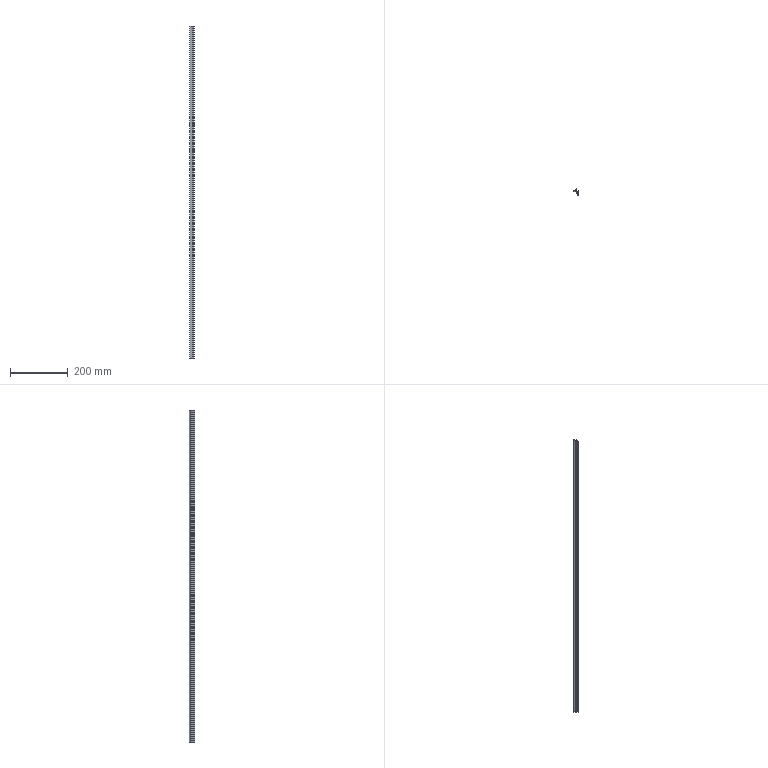Part | SolidWorks | features BaseBody 1, ICE 1, MoveFace 1 | 1 solid | 27 faces | box 14 x 20.3 x 1150 mm | volume 58553 mm3 | plane 20 | cylinder 7 | commonest cylinder face diameters 0.387 x2 0.8 x2 0.4 x1 20 x1 22 x1
STEP:
#1=CARTESIAN_POINT('',(-5.304,-0.625,200.));
#2=VERTEX_POINT('',#1);
#3=CARTESIAN_POINT('',(-5.449,-0.8125,200.));
#4=VERTEX_POINT('',#3);
#5=CARTESIAN_POINT('',(-5.255,-0.8125,200.));
#6=DIRECTION('',(0.,0.,1.));
#7=DIRECTION('',(-1.,0.,0.));
#8=AXIS2_PLACEMENT_3D('',#5,#6,#7);
#9=CIRCLE('',#8,0.1937);
#10=EDGE_CURVE('',#2,#4,#9,.T.);
#11=ORIENTED_EDGE('',*,*,#10,.T.);
#12=CARTESIAN_POINT('',(-5.449,-0.8125,-950.));
#13=VERTEX_POINT('',#12);
#14=CARTESIAN_POINT('',(-5.449,-0.8125,230.));
#15=DIRECTION('',(0.,0.,-1.));
#16=VECTOR('',#15,1000.);
#17=LINE('',#14,#16);
#18=EDGE_CURVE('',#4,#13,#17,.T.);
#19=ORIENTED_EDGE('',*,*,#18,.T.);
#20=CARTESIAN_POINT('',(-5.304,-0.625,-950.));
#21=VERTEX_POINT('',#20);
#22=CARTESIAN_POINT('',(-5.255,-0.8125,-950.));
#23=DIRECTION('',(0.,0.,-1.));
#24=DIRECTION('',(1.,0.,0.));
#25=AXIS2_PLACEMENT_3D('',#22,#23,#24);
#26=CIRCLE('',#25,0.1937);
#27=EDGE_CURVE('',#13,#21,#26,.T.);
#28=ORIENTED_EDGE('',*,*,#27,.T.);
#29=CARTESIAN_POINT('',(-5.304,-0.625,230.));
#30=DIRECTION('',(0.,0.,-1.));
#31=VECTOR('',#30,1000.);
#32=LINE('',#29,#31);
#33=EDGE_CURVE('',#2,#21,#32,.T.);
#34=ORIENTED_EDGE('',*,*,#33,.F.);
#35=EDGE_LOOP('',(#11,#19,#28,#34));
#36=FACE_OUTER_BOUND('',#35,.T.);
#37=CARTESIAN_POINT('',(-5.255,-0.8125,230.));
#38=DIRECTION('',(0.,0.,-1.));
#39=DIRECTION('',(-1.,0.,0.));
#40=AXIS2_PLACEMENT_3D('',#37,#38,#39);
#41=CYLINDRICAL_SURFACE('',#40,0.1937);
#42=ADVANCED_FACE('',(#36),#41,.F.);
#43=CARTESIAN_POINT('',(5.,-1.,-950.));
#44=VERTEX_POINT('',#43);
#45=CARTESIAN_POINT('',(5.,-14.3,-950.));
#46=VERTEX_POINT('',#45);
#47=CARTESIAN_POINT('',(5.,29.623,-950.));
#48=DIRECTION('',(0.,-1.,0.));
#49=VECTOR('',#48,1000.);
#50=LINE('',#47,#49);
#51=EDGE_CURVE('',#44,#46,#50,.T.);
#52=ORIENTED_EDGE('',*,*,#51,.F.);
#53=CARTESIAN_POINT('',(5.,-1.,200.));
#54=VERTEX_POINT('',#53);
#55=CARTESIAN_POINT('',(5.,-1.,230.));
#56=DIRECTION('',(0.,0.,-1.));
#57=VECTOR('',#56,1000.);
#58=LINE('',#55,#57);
#59=EDGE_CURVE('',#54,#44,#58,.T.);
#60=ORIENTED_EDGE('',*,*,#59,.F.);
#61=CARTESIAN_POINT('',(5.,-14.3,200.));
#62=VERTEX_POINT('',#61);
#63=CARTESIAN_POINT('',(5.,-14.3,200.));
#64=DIRECTION('',(0.,1.,0.));
#65=VECTOR('',#64,1000.);
#66=LINE('',#63,#65);
#67=EDGE_CURVE('',#62,#54,#66,.T.);
#68=ORIENTED_EDGE('',*,*,#67,.F.);
#69=CARTESIAN_POINT('',(5.,-14.3,230.));
#70=DIRECTION('',(0.,0.,1.));
#71=VECTOR('',#70,1000.);
#72=LINE('',#69,#71);
#73=EDGE_CURVE('',#46,#62,#72,.T.);
#74=ORIENTED_EDGE('',*,*,#73,.F.);
#75=EDGE_LOOP('',(#52,#60,#68,#74));
#76=FACE_OUTER_BOUND('',#75,.T.);
#77=CARTESIAN_POINT('',(5.,-14.3,230.));
#78=DIRECTION('',(-1.,0.,0.));
#79=DIRECTION('',(0.,0.,1.));
#80=AXIS2_PLACEMENT_3D('',#77,#78,#79);
#81=PLANE('',#80);
#82=ADVANCED_FACE('',(#76),#81,.F.);
#83=CARTESIAN_POINT('',(-9.,-2.,-950.));
#84=VERTEX_POINT('',#83);
#85=CARTESIAN_POINT('',(-9.,-2.,200.));
#86=VERTEX_POINT('',#85);
#87=CARTESIAN_POINT('',(-9.,-2.,230.));
#88=DIRECTION('',(0.,0.,1.));
#89=VECTOR('',#88,1000.);
#90=LINE('',#87,#89);
#91=EDGE_CURVE('',#84,#86,#90,.T.);
#92=ORIENTED_EDGE('',*,*,#91,.F.);
#93=CARTESIAN_POINT('',(0.9,-2.,-950.));
#94=VERTEX_POINT('',#93);
#95=CARTESIAN_POINT('',(5.,-2.,-950.));
#96=DIRECTION('',(-1.,0.,0.));
#97=VECTOR('',#96,1000.);
#98=LINE('',#95,#97);
#99=EDGE_CURVE('',#94,#84,#98,.T.);
#100=ORIENTED_EDGE('',*,*,#99,.F.);
#101=CARTESIAN_POINT('',(0.9,-2.,200.));
#102=VERTEX_POINT('',#101);
#103=CARTESIAN_POINT('',(0.9,-2.,230.));
#104=DIRECTION('',(0.,0.,-1.));
#105=VECTOR('',#104,1000.);
#106=LINE('',#103,#105);
#107=EDGE_CURVE('',#102,#94,#106,.T.);
#108=ORIENTED_EDGE('',*,*,#107,.F.);
#109=CARTESIAN_POINT('',(5.,-2.,200.));
#110=DIRECTION('',(1.,0.,0.));
#111=VECTOR('',#110,1000.);
#112=LINE('',#109,#111);
#113=EDGE_CURVE('',#86,#102,#112,.T.);
#114=ORIENTED_EDGE('',*,*,#113,.F.);
#115=EDGE_LOOP('',(#92,#100,#108,#114));
#116=FACE_OUTER_BOUND('',#115,.T.);
#117=CARTESIAN_POINT('',(-9.,-2.,230.));
#118=DIRECTION('',(0.,1.,0.));
#119=DIRECTION('',(0.,0.,1.));
#120=AXIS2_PLACEMENT_3D('',#117,#118,#119);
#121=PLANE('',#120);
#122=ADVANCED_FACE('',(#116),#121,.F.);
#123=CARTESIAN_POINT('',(4.,-6.,200.));
#124=VERTEX_POINT('',#123);
#125=CARTESIAN_POINT('',(4.,-3.,200.));
#126=VERTEX_POINT('',#125);
#127=CARTESIAN_POINT('',(4.,29.623,200.));
#128=DIRECTION('',(0.,1.,0.));
#129=VECTOR('',#128,1000.);
#130=LINE('',#127,#129);
#131=EDGE_CURVE('',#124,#126,#130,.T.);
#132=ORIENTED_EDGE('',*,*,#131,.F.);
#133=CARTESIAN_POINT('',(1.,-6.,200.));
#134=VERTEX_POINT('',#133);
#135=CARTESIAN_POINT('',(5.,-6.,200.));
#136=DIRECTION('',(1.,0.,0.));
#137=VECTOR('',#136,1000.);
#138=LINE('',#135,#137);
#139=EDGE_CURVE('',#134,#124,#138,.T.);
#140=ORIENTED_EDGE('',*,*,#139,.F.);
#141=CARTESIAN_POINT('',(1.,-6.7,200.));
#142=VERTEX_POINT('',#141);
#143=CARTESIAN_POINT('',(1.,-6.,200.));
#144=DIRECTION('',(0.,-1.,0.));
#145=VECTOR('',#144,1000.);
#146=LINE('',#143,#145);
#147=EDGE_CURVE('',#134,#142,#146,.T.);
#148=ORIENTED_EDGE('',*,*,#147,.T.);
#149=CARTESIAN_POINT('',(-1.7,-6.7,200.));
#150=VERTEX_POINT('',#149);
#151=CARTESIAN_POINT('',(5.,-6.7,200.));
#152=DIRECTION('',(1.,0.,0.));
#153=VECTOR('',#152,1000.);
#154=LINE('',#151,#153);
#155=EDGE_CURVE('',#150,#142,#154,.T.);
#156=ORIENTED_EDGE('',*,*,#155,.F.);
#157=CARTESIAN_POINT('',(-1.7,-7.7,200.));
#158=VERTEX_POINT('',#157);
#159=CARTESIAN_POINT('',(-1.7,-6.7,200.));
#160=DIRECTION('',(0.,-1.,0.));
#161=VECTOR('',#160,1000.);
#162=LINE('',#159,#161);
#163=EDGE_CURVE('',#150,#158,#162,.T.);
#164=ORIENTED_EDGE('',*,*,#163,.T.);
#165=CARTESIAN_POINT('',(4.,-7.7,200.));
#166=VERTEX_POINT('',#165);
#167=CARTESIAN_POINT('',(5.,-7.7,200.));
#168=DIRECTION('',(-1.,0.,0.));
#169=VECTOR('',#168,1000.);
#170=LINE('',#167,#169);
#171=EDGE_CURVE('',#166,#158,#170,.T.);
#172=ORIENTED_EDGE('',*,*,#171,.F.);
#173=CARTESIAN_POINT('',(4.,-14.3,200.));
#174=VERTEX_POINT('',#173);
#175=CARTESIAN_POINT('',(4.,29.623,200.));
#176=DIRECTION('',(0.,1.,0.));
#177=VECTOR('',#176,1000.);
#178=LINE('',#175,#177);
#179=EDGE_CURVE('',#174,#166,#178,.T.);
#180=ORIENTED_EDGE('',*,*,#179,.F.);
#181=CARTESIAN_POINT('',(5.,-14.3,200.));
#182=DIRECTION('',(-1.,0.,0.));
#183=VECTOR('',#182,1000.);
#184=LINE('',#181,#183);
#185=EDGE_CURVE('',#62,#174,#184,.T.);
#186=ORIENTED_EDGE('',*,*,#185,.F.);
#187=ORIENTED_EDGE('',*,*,#67,.T.);
#188=CARTESIAN_POINT('',(-5.207,-1.,200.));
#189=VERTEX_POINT('',#188);
#190=CARTESIAN_POINT('',(5.,-1.,200.));
#191=DIRECTION('',(1.,0.,0.));
#192=VECTOR('',#191,1000.);
#193=LINE('',#190,#192);
#194=EDGE_CURVE('',#189,#54,#193,.T.);
#195=ORIENTED_EDGE('',*,*,#194,.F.);
#196=CARTESIAN_POINT('',(-5.255,-0.8125,200.));
#197=DIRECTION('',(0.,0.,1.));
#198=DIRECTION('',(-1.,0.,0.));
#199=AXIS2_PLACEMENT_3D('',#196,#197,#198);
#200=CIRCLE('',#199,0.1937);
#201=EDGE_CURVE('',#4,#189,#200,.T.);
#202=ORIENTED_EDGE('',*,*,#201,.F.);
#203=ORIENTED_EDGE('',*,*,#10,.F.);
#204=CARTESIAN_POINT('',(-1.368,3.063,200.));
#205=VERTEX_POINT('',#204);
#206=CARTESIAN_POINT('',(-10.628,9.,200.));
#207=DIRECTION('',(0.,0.,1.));
#208=DIRECTION('',(-1.,0.,0.));
#209=AXIS2_PLACEMENT_3D('',#206,#207,#208);
#210=CIRCLE('',#209,11.);
#211=EDGE_CURVE('',#2,#205,#210,.T.);
#212=ORIENTED_EDGE('',*,*,#211,.T.);
#213=CARTESIAN_POINT('',(-1.,2.955,200.));
#214=VERTEX_POINT('',#213);
#215=CARTESIAN_POINT('',(-1.2,2.955,200.));
#216=DIRECTION('',(0.,0.,1.));
#217=DIRECTION('',(-1.,0.,0.));
#218=AXIS2_PLACEMENT_3D('',#215,#216,#217);
#219=CIRCLE('',#218,0.2);
#220=EDGE_CURVE('',#214,#205,#219,.T.);
#221=ORIENTED_EDGE('',*,*,#220,.F.);
#222=CARTESIAN_POINT('',(-1.,1.5,200.));
#223=VERTEX_POINT('',#222);
#224=CARTESIAN_POINT('',(-1.,2.955,200.));
#225=DIRECTION('',(0.,1.,0.));
#226=VECTOR('',#225,1000.);
#227=LINE('',#224,#226);
#228=EDGE_CURVE('',#223,#214,#227,.T.);
#229=ORIENTED_EDGE('',*,*,#228,.F.);
#230=CARTESIAN_POINT('',(0.,1.5,200.));
#231=VERTEX_POINT('',#230);
#232=CARTESIAN_POINT('',(-1.,1.5,200.));
#233=DIRECTION('',(-1.,0.,0.));
#234=VECTOR('',#233,1000.);
#235=LINE('',#232,#234);
#236=EDGE_CURVE('',#231,#223,#235,.T.);
#237=ORIENTED_EDGE('',*,*,#236,.F.);
#238=CARTESIAN_POINT('',(0.,6.,200.));
#239=VERTEX_POINT('',#238);
#240=CARTESIAN_POINT('',(0.,1.5,200.));
#241=DIRECTION('',(0.,-1.,0.));
#242=VECTOR('',#241,1000.);
#243=LINE('',#240,#242);
#244=EDGE_CURVE('',#239,#231,#243,.T.);
#245=ORIENTED_EDGE('',*,*,#244,.F.);
#246=CARTESIAN_POINT('',(-0.8,6.,200.));
#247=VERTEX_POINT('',#246);
#248=CARTESIAN_POINT('',(0.,6.,200.));
#249=DIRECTION('',(1.,0.,0.));
#250=VECTOR('',#249,1000.);
#251=LINE('',#248,#250);
#252=EDGE_CURVE('',#247,#239,#251,.T.);
#253=ORIENTED_EDGE('',*,*,#252,.F.);
#254=CARTESIAN_POINT('',(-1.178,5.731,200.));
#255=VERTEX_POINT('',#254);
#256=CARTESIAN_POINT('',(-0.8,5.6,200.));
#257=DIRECTION('',(0.,0.,1.));
#258=DIRECTION('',(-1.,0.,0.));
#259=AXIS2_PLACEMENT_3D('',#256,#257,#258);
#260=CIRCLE('',#259,0.4);
#261=EDGE_CURVE('',#247,#255,#260,.T.);
#262=ORIENTED_EDGE('',*,*,#261,.T.);
#263=CARTESIAN_POINT('',(-8.678,-0.8077,200.));
#264=VERTEX_POINT('',#263);
#265=CARTESIAN_POINT('',(-10.628,9.,200.));
#266=DIRECTION('',(0.,0.,1.));
#267=DIRECTION('',(-1.,0.,0.));
#268=AXIS2_PLACEMENT_3D('',#265,#266,#267);
#269=CIRCLE('',#268,10.);
#270=EDGE_CURVE('',#264,#255,#269,.T.);
#271=ORIENTED_EDGE('',*,*,#270,.F.);
#272=CARTESIAN_POINT('',(-9.,-1.2,200.));
#273=VERTEX_POINT('',#272);
#274=CARTESIAN_POINT('',(-8.6,-1.2,200.));
#275=DIRECTION('',(0.,0.,1.));
#276=DIRECTION('',(-1.,0.,0.));
#277=AXIS2_PLACEMENT_3D('',#274,#275,#276);
#278=CIRCLE('',#277,0.4);
#279=EDGE_CURVE('',#264,#273,#278,.T.);
#280=ORIENTED_EDGE('',*,*,#279,.T.);
#281=CARTESIAN_POINT('',(-9.,8.,200.));
#282=DIRECTION('',(0.,-1.,0.));
#283=VECTOR('',#282,1000.);
#284=LINE('',#281,#283);
#285=EDGE_CURVE('',#273,#86,#284,.T.);
#286=ORIENTED_EDGE('',*,*,#285,.T.);
#287=ORIENTED_EDGE('',*,*,#113,.T.);
#288=CARTESIAN_POINT('',(0.9,-3.,200.));
#289=VERTEX_POINT('',#288);
#290=CARTESIAN_POINT('',(0.9,29.623,200.));
#291=DIRECTION('',(0.,1.,0.));
#292=VECTOR('',#291,1000.);
#293=LINE('',#290,#292);
#294=EDGE_CURVE('',#289,#102,#293,.T.);
#295=ORIENTED_EDGE('',*,*,#294,.F.);
#296=CARTESIAN_POINT('',(5.,-3.,200.));
#297=DIRECTION('',(-1.,0.,0.));
#298=VECTOR('',#297,1000.);
#299=LINE('',#296,#298);
#300=EDGE_CURVE('',#126,#289,#299,.T.);
#301=ORIENTED_EDGE('',*,*,#300,.F.);
#302=EDGE_LOOP('',(#132,#140,#148,#156,#164,#172,#180,#186,#187,#195,#202,#203,#212,#221,#229,#237,#245,#253,#262,#271,#280,#286,#287,#295,#301));
#303=FACE_OUTER_BOUND('',#302,.T.);
#304=CARTESIAN_POINT('',(5.,29.623,200.));
#305=DIRECTION('',(0.,0.,-1.));
#306=DIRECTION('',(-1.,0.,0.));
#307=AXIS2_PLACEMENT_3D('',#304,#305,#306);
#308=PLANE('',#307);
#309=ADVANCED_FACE('',(#303),#308,.F.);
#310=ORIENTED_EDGE('',*,*,#185,.T.);
#311=CARTESIAN_POINT('',(4.,-14.3,-950.));
#312=VERTEX_POINT('',#311);
#313=CARTESIAN_POINT('',(4.,-14.3,230.));
#314=DIRECTION('',(0.,0.,1.));
#315=VECTOR('',#314,1000.);
#316=LINE('',#313,#315);
#317=EDGE_CURVE('',#312,#174,#316,.T.);
#318=ORIENTED_EDGE('',*,*,#317,.F.);
#319=CARTESIAN_POINT('',(5.,-14.3,-950.));
#320=DIRECTION('',(-1.,0.,0.));
#321=VECTOR('',#320,1000.);
#322=LINE('',#319,#321);
#323=EDGE_CURVE('',#46,#312,#322,.T.);
#324=ORIENTED_EDGE('',*,*,#323,.F.);
#325=ORIENTED_EDGE('',*,*,#73,.T.);
#326=EDGE_LOOP('',(#310,#318,#324,#325));
#327=FACE_OUTER_BOUND('',#326,.T.);
#328=CARTESIAN_POINT('',(4.,-14.3,230.));
#329=DIRECTION('',(0.,1.,0.));
#330=DIRECTION('',(0.,0.,1.));
#331=AXIS2_PLACEMENT_3D('',#328,#329,#330);
#332=PLANE('',#331);
#333=ADVANCED_FACE('',(#327),#332,.F.);
#334=ORIENTED_EDGE('',*,*,#51,.T.);
#335=ORIENTED_EDGE('',*,*,#323,.T.);
#336=CARTESIAN_POINT('',(4.,-7.7,-950.));
#337=VERTEX_POINT('',#336);
#338=CARTESIAN_POINT('',(4.,-7.7,-950.));
#339=DIRECTION('',(0.,-1.,0.));
#340=VECTOR('',#339,1000.);
#341=LINE('',#338,#340);
#342=EDGE_CURVE('',#337,#312,#341,.T.);
#343=ORIENTED_EDGE('',*,*,#342,.F.);
#344=CARTESIAN_POINT('',(-1.7,-7.7,-950.));
#345=VERTEX_POINT('',#344);
#346=CARTESIAN_POINT('',(-1.7,-7.7,-950.));
#347=DIRECTION('',(1.,0.,0.));
#348=VECTOR('',#347,1000.);
#349=LINE('',#346,#348);
#350=EDGE_CURVE('',#345,#337,#349,.T.);
#351=ORIENTED_EDGE('',*,*,#350,.F.);
#352=CARTESIAN_POINT('',(-1.7,-6.7,-950.));
#353=VERTEX_POINT('',#352);
#354=CARTESIAN_POINT('',(-1.7,29.623,-950.));
#355=DIRECTION('',(0.,1.,0.));
#356=VECTOR('',#355,1000.);
#357=LINE('',#354,#356);
#358=EDGE_CURVE('',#345,#353,#357,.T.);
#359=ORIENTED_EDGE('',*,*,#358,.T.);
#360=CARTESIAN_POINT('',(1.,-6.7,-950.));
#361=VERTEX_POINT('',#360);
#362=CARTESIAN_POINT('',(1.,-6.7,-950.));
#363=DIRECTION('',(-1.,0.,0.));
#364=VECTOR('',#363,1000.);
#365=LINE('',#362,#364);
#366=EDGE_CURVE('',#361,#353,#365,.T.);
#367=ORIENTED_EDGE('',*,*,#366,.F.);
#368=CARTESIAN_POINT('',(1.,-6.,-950.));
#369=VERTEX_POINT('',#368);
#370=CARTESIAN_POINT('',(1.,29.623,-950.));
#371=DIRECTION('',(0.,1.,0.));
#372=VECTOR('',#371,1000.);
#373=LINE('',#370,#372);
#374=EDGE_CURVE('',#361,#369,#373,.T.);
#375=ORIENTED_EDGE('',*,*,#374,.T.);
#376=CARTESIAN_POINT('',(4.,-6.,-950.));
#377=VERTEX_POINT('',#376);
#378=CARTESIAN_POINT('',(4.,-6.,-950.));
#379=DIRECTION('',(-1.,0.,0.));
#380=VECTOR('',#379,1000.);
#381=LINE('',#378,#380);
#382=EDGE_CURVE('',#377,#369,#381,.T.);
#383=ORIENTED_EDGE('',*,*,#382,.F.);
#384=CARTESIAN_POINT('',(4.,-3.,-950.));
#385=VERTEX_POINT('',#384);
#386=CARTESIAN_POINT('',(4.,-3.,-950.));
#387=DIRECTION('',(0.,-1.,0.));
#388=VECTOR('',#387,1000.);
#389=LINE('',#386,#388);
#390=EDGE_CURVE('',#385,#377,#389,.T.);
#391=ORIENTED_EDGE('',*,*,#390,.F.);
#392=CARTESIAN_POINT('',(0.9,-3.,-950.));
#393=VERTEX_POINT('',#392);
#394=CARTESIAN_POINT('',(0.9,-3.,-950.));
#395=DIRECTION('',(1.,0.,0.));
#396=VECTOR('',#395,1000.);
#397=LINE('',#394,#396);
#398=EDGE_CURVE('',#393,#385,#397,.T.);
#399=ORIENTED_EDGE('',*,*,#398,.F.);
#400=CARTESIAN_POINT('',(0.9,-2.,-950.));
#401=DIRECTION('',(0.,-1.,0.));
#402=VECTOR('',#401,1000.);
#403=LINE('',#400,#402);
#404=EDGE_CURVE('',#94,#393,#403,.T.);
#405=ORIENTED_EDGE('',*,*,#404,.F.);
#406=ORIENTED_EDGE('',*,*,#99,.T.);
#407=CARTESIAN_POINT('',(-9.,-1.2,-950.));
#408=VERTEX_POINT('',#407);
#409=CARTESIAN_POINT('',(-9.,-1.2,-950.));
#410=DIRECTION('',(0.,-1.,0.));
#411=VECTOR('',#410,1000.);
#412=LINE('',#409,#411);
#413=EDGE_CURVE('',#408,#84,#412,.T.);
#414=ORIENTED_EDGE('',*,*,#413,.F.);
#415=CARTESIAN_POINT('',(-8.678,-0.8077,-950.));
#416=VERTEX_POINT('',#415);
#417=CARTESIAN_POINT('',(-8.6,-1.2,-950.));
#418=DIRECTION('',(0.,0.,-1.));
#419=DIRECTION('',(1.,0.,0.));
#420=AXIS2_PLACEMENT_3D('',#417,#418,#419);
#421=CIRCLE('',#420,0.4);
#422=EDGE_CURVE('',#408,#416,#421,.T.);
#423=ORIENTED_EDGE('',*,*,#422,.T.);
#424=CARTESIAN_POINT('',(-1.178,5.731,-950.));
#425=VERTEX_POINT('',#424);
#426=CARTESIAN_POINT('',(-10.628,9.,-950.));
#427=DIRECTION('',(0.,0.,-1.));
#428=DIRECTION('',(1.,0.,0.));
#429=AXIS2_PLACEMENT_3D('',#426,#427,#428);
#430=CIRCLE('',#429,10.);
#431=EDGE_CURVE('',#425,#416,#430,.T.);
#432=ORIENTED_EDGE('',*,*,#431,.F.);
#433=CARTESIAN_POINT('',(-0.8,6.,-950.));
#434=VERTEX_POINT('',#433);
#435=CARTESIAN_POINT('',(-0.8,5.6,-950.));
#436=DIRECTION('',(0.,0.,-1.));
#437=DIRECTION('',(1.,0.,0.));
#438=AXIS2_PLACEMENT_3D('',#435,#436,#437);
#439=CIRCLE('',#438,0.4);
#440=EDGE_CURVE('',#425,#434,#439,.T.);
#441=ORIENTED_EDGE('',*,*,#440,.T.);
#442=CARTESIAN_POINT('',(0.,6.,-950.));
#443=VERTEX_POINT('',#442);
#444=CARTESIAN_POINT('',(0.,6.,-950.));
#445=DIRECTION('',(-1.,0.,0.));
#446=VECTOR('',#445,1000.);
#447=LINE('',#444,#446);
#448=EDGE_CURVE('',#443,#434,#447,.T.);
#449=ORIENTED_EDGE('',*,*,#448,.F.);
#450=CARTESIAN_POINT('',(0.,1.5,-950.));
#451=VERTEX_POINT('',#450);
#452=CARTESIAN_POINT('',(0.,1.5,-950.));
#453=DIRECTION('',(0.,1.,0.));
#454=VECTOR('',#453,1000.);
#455=LINE('',#452,#454);
#456=EDGE_CURVE('',#451,#443,#455,.T.);
#457=ORIENTED_EDGE('',*,*,#456,.F.);
#458=CARTESIAN_POINT('',(-1.,1.5,-950.));
#459=VERTEX_POINT('',#458);
#460=CARTESIAN_POINT('',(-1.,1.5,-950.));
#461=DIRECTION('',(1.,0.,0.));
#462=VECTOR('',#461,1000.);
#463=LINE('',#460,#462);
#464=EDGE_CURVE('',#459,#451,#463,.T.);
#465=ORIENTED_EDGE('',*,*,#464,.F.);
#466=CARTESIAN_POINT('',(-1.,2.955,-950.));
#467=VERTEX_POINT('',#466);
#468=CARTESIAN_POINT('',(-1.,2.955,-950.));
#469=DIRECTION('',(0.,-1.,0.));
#470=VECTOR('',#469,1000.);
#471=LINE('',#468,#470);
#472=EDGE_CURVE('',#467,#459,#471,.T.);
#473=ORIENTED_EDGE('',*,*,#472,.F.);
#474=CARTESIAN_POINT('',(-1.368,3.063,-950.));
#475=VERTEX_POINT('',#474);
#476=CARTESIAN_POINT('',(-1.2,2.955,-950.));
#477=DIRECTION('',(0.,0.,-1.));
#478=DIRECTION('',(1.,0.,0.));
#479=AXIS2_PLACEMENT_3D('',#476,#477,#478);
#480=CIRCLE('',#479,0.2);
#481=EDGE_CURVE('',#475,#467,#480,.T.);
#482=ORIENTED_EDGE('',*,*,#481,.F.);
#483=CARTESIAN_POINT('',(-10.628,9.,-950.));
#484=DIRECTION('',(0.,0.,-1.));
#485=DIRECTION('',(1.,0.,0.));
#486=AXIS2_PLACEMENT_3D('',#483,#484,#485);
#487=CIRCLE('',#486,11.);
#488=EDGE_CURVE('',#475,#21,#487,.T.);
#489=ORIENTED_EDGE('',*,*,#488,.T.);
#490=ORIENTED_EDGE('',*,*,#27,.F.);
#491=CARTESIAN_POINT('',(-5.207,-1.,-950.));
#492=VERTEX_POINT('',#491);
#493=CARTESIAN_POINT('',(-5.255,-0.8125,-950.));
#494=DIRECTION('',(0.,0.,-1.));
#495=DIRECTION('',(1.,0.,0.));
#496=AXIS2_PLACEMENT_3D('',#493,#494,#495);
#497=CIRCLE('',#496,0.1937);
#498=EDGE_CURVE('',#492,#13,#497,.T.);
#499=ORIENTED_EDGE('',*,*,#498,.F.);
#500=CARTESIAN_POINT('',(5.,-1.,-950.));
#501=DIRECTION('',(-1.,0.,0.));
#502=VECTOR('',#501,1000.);
#503=LINE('',#500,#502);
#504=EDGE_CURVE('',#44,#492,#503,.T.);
#505=ORIENTED_EDGE('',*,*,#504,.F.);
#506=EDGE_LOOP('',(#334,#335,#343,#351,#359,#367,#375,#383,#391,#399,#405,#406,#414,#423,#432,#441,#449,#457,#465,#473,#482,#489,#490,#499,#505));
#507=FACE_OUTER_BOUND('',#506,.T.);
#508=CARTESIAN_POINT('',(5.,29.623,-950.));
#509=DIRECTION('',(0.,0.,1.));
#510=DIRECTION('',(1.,0.,0.));
#511=AXIS2_PLACEMENT_3D('',#508,#509,#510);
#512=PLANE('',#511);
#513=ADVANCED_FACE('',(#507),#512,.F.);
#514=ORIENTED_EDGE('',*,*,#59,.T.);
#515=ORIENTED_EDGE('',*,*,#504,.T.);
#516=CARTESIAN_POINT('',(-5.207,-1.,230.));
#517=DIRECTION('',(0.,0.,-1.));
#518=VECTOR('',#517,1000.);
#519=LINE('',#516,#518);
#520=EDGE_CURVE('',#189,#492,#519,.T.);
#521=ORIENTED_EDGE('',*,*,#520,.F.);
#522=ORIENTED_EDGE('',*,*,#194,.T.);
#523=EDGE_LOOP('',(#514,#515,#521,#522));
#524=FACE_OUTER_BOUND('',#523,.T.);
#525=CARTESIAN_POINT('',(5.,-1.,230.));
#526=DIRECTION('',(0.,-1.,0.));
#527=DIRECTION('',(0.,0.,-1.));
#528=AXIS2_PLACEMENT_3D('',#525,#526,#527);
#529=PLANE('',#528);
#530=ADVANCED_FACE('',(#524),#529,.F.);
#531=CARTESIAN_POINT('',(-9.,-1.2,230.));
#532=DIRECTION('',(0.,0.,1.));
#533=VECTOR('',#532,1000.);
#534=LINE('',#531,#533);
#535=EDGE_CURVE('',#408,#273,#534,.T.);
#536=ORIENTED_EDGE('',*,*,#535,.F.);
#537=ORIENTED_EDGE('',*,*,#413,.T.);
#538=ORIENTED_EDGE('',*,*,#91,.T.);
#539=ORIENTED_EDGE('',*,*,#285,.F.);
#540=EDGE_LOOP('',(#536,#537,#538,#539));
#541=FACE_OUTER_BOUND('',#540,.T.);
#542=CARTESIAN_POINT('',(-9.,-1.2,230.));
#543=DIRECTION('',(1.,0.,0.));
#544=DIRECTION('',(0.,0.,-1.));
#545=AXIS2_PLACEMENT_3D('',#542,#543,#544);
#546=PLANE('',#545);
#547=ADVANCED_FACE('',(#541),#546,.F.);
#548=ORIENTED_EDGE('',*,*,#294,.T.);
#549=ORIENTED_EDGE('',*,*,#107,.T.);
#550=ORIENTED_EDGE('',*,*,#404,.T.);
#551=CARTESIAN_POINT('',(0.9,-3.,230.));
#552=DIRECTION('',(0.,0.,-1.));
#553=VECTOR('',#552,1000.);
#554=LINE('',#551,#553);
#555=EDGE_CURVE('',#289,#393,#554,.T.);
#556=ORIENTED_EDGE('',*,*,#555,.F.);
#557=EDGE_LOOP('',(#548,#549,#550,#556));
#558=FACE_OUTER_BOUND('',#557,.T.);
#559=CARTESIAN_POINT('',(0.9,-2.,230.));
#560=DIRECTION('',(1.,0.,0.));
#561=DIRECTION('',(0.,0.,-1.));
#562=AXIS2_PLACEMENT_3D('',#559,#560,#561);
#563=PLANE('',#562);
#564=ADVANCED_FACE('',(#558),#563,.F.);
#565=ORIENTED_EDGE('',*,*,#300,.T.);
#566=ORIENTED_EDGE('',*,*,#555,.T.);
#567=ORIENTED_EDGE('',*,*,#398,.T.);
#568=CARTESIAN_POINT('',(4.,-3.,230.));
#569=DIRECTION('',(0.,0.,-1.));
#570=VECTOR('',#569,1000.);
#571=LINE('',#568,#570);
#572=EDGE_CURVE('',#126,#385,#571,.T.);
#573=ORIENTED_EDGE('',*,*,#572,.F.);
#574=EDGE_LOOP('',(#565,#566,#567,#573));
#575=FACE_OUTER_BOUND('',#574,.T.);
#576=CARTESIAN_POINT('',(0.9,-3.,230.));
#577=DIRECTION('',(0.,1.,0.));
#578=DIRECTION('',(0.,0.,1.));
#579=AXIS2_PLACEMENT_3D('',#576,#577,#578);
#580=PLANE('',#579);
#581=ADVANCED_FACE('',(#575),#580,.F.);
#582=ORIENTED_EDGE('',*,*,#131,.T.);
#583=ORIENTED_EDGE('',*,*,#572,.T.);
#584=ORIENTED_EDGE('',*,*,#390,.T.);
#585=CARTESIAN_POINT('',(4.,-6.,230.));
#586=DIRECTION('',(0.,0.,-1.));
#587=VECTOR('',#586,1000.);
#588=LINE('',#585,#587);
#589=EDGE_CURVE('',#124,#377,#588,.T.);
#590=ORIENTED_EDGE('',*,*,#589,.F.);
#591=EDGE_LOOP('',(#582,#583,#584,#590));
#592=FACE_OUTER_BOUND('',#591,.T.);
#593=CARTESIAN_POINT('',(4.,-3.,230.));
#594=DIRECTION('',(1.,0.,0.));
#595=DIRECTION('',(0.,0.,-1.));
#596=AXIS2_PLACEMENT_3D('',#593,#594,#595);
#597=PLANE('',#596);
#598=ADVANCED_FACE('',(#592),#597,.F.);
#599=ORIENTED_EDGE('',*,*,#139,.T.);
#600=ORIENTED_EDGE('',*,*,#589,.T.);
#601=ORIENTED_EDGE('',*,*,#382,.T.);
#602=CARTESIAN_POINT('',(1.,-6.,230.));
#603=DIRECTION('',(0.,0.,-1.));
#604=VECTOR('',#603,1000.);
#605=LINE('',#602,#604);
#606=EDGE_CURVE('',#134,#369,#605,.T.);
#607=ORIENTED_EDGE('',*,*,#606,.F.);
#608=EDGE_LOOP('',(#599,#600,#601,#607));
#609=FACE_OUTER_BOUND('',#608,.T.);
#610=CARTESIAN_POINT('',(4.,-6.,230.));
#611=DIRECTION('',(0.,-1.,0.));
#612=DIRECTION('',(0.,0.,-1.));
#613=AXIS2_PLACEMENT_3D('',#610,#611,#612);
#614=PLANE('',#613);
#615=ADVANCED_FACE('',(#609),#614,.F.);
#616=ORIENTED_EDGE('',*,*,#155,.T.);
#617=CARTESIAN_POINT('',(1.,-6.7,230.));
#618=DIRECTION('',(0.,0.,1.));
#619=VECTOR('',#618,1000.);
#620=LINE('',#617,#619);
#621=EDGE_CURVE('',#361,#142,#620,.T.);
#622=ORIENTED_EDGE('',*,*,#621,.F.);
#623=ORIENTED_EDGE('',*,*,#366,.T.);
#624=CARTESIAN_POINT('',(-1.7,-6.7,230.));
#625=DIRECTION('',(0.,0.,-1.));
#626=VECTOR('',#625,1000.);
#627=LINE('',#624,#626);
#628=EDGE_CURVE('',#150,#353,#627,.T.);
#629=ORIENTED_EDGE('',*,*,#628,.F.);
#630=EDGE_LOOP('',(#616,#622,#623,#629));
#631=FACE_OUTER_BOUND('',#630,.T.);
#632=CARTESIAN_POINT('',(1.,-6.7,230.));
#633=DIRECTION('',(0.,-1.,0.));
#634=DIRECTION('',(0.,0.,-1.));
#635=AXIS2_PLACEMENT_3D('',#632,#633,#634);
#636=PLANE('',#635);
#637=ADVANCED_FACE('',(#631),#636,.F.);
#638=ORIENTED_EDGE('',*,*,#171,.T.);
#639=CARTESIAN_POINT('',(-1.7,-7.7,230.));
#640=DIRECTION('',(0.,0.,1.));
#641=VECTOR('',#640,1000.);
#642=LINE('',#639,#641);
#643=EDGE_CURVE('',#345,#158,#642,.T.);
#644=ORIENTED_EDGE('',*,*,#643,.F.);
#645=ORIENTED_EDGE('',*,*,#350,.T.);
#646=CARTESIAN_POINT('',(4.,-7.7,230.));
#647=DIRECTION('',(0.,0.,-1.));
#648=VECTOR('',#647,1000.);
#649=LINE('',#646,#648);
#650=EDGE_CURVE('',#166,#337,#649,.T.);
#651=ORIENTED_EDGE('',*,*,#650,.F.);
#652=EDGE_LOOP('',(#638,#644,#645,#651));
#653=FACE_OUTER_BOUND('',#652,.T.);
#654=CARTESIAN_POINT('',(-1.7,-7.7,230.));
#655=DIRECTION('',(0.,1.,0.));
#656=DIRECTION('',(0.,0.,1.));
#657=AXIS2_PLACEMENT_3D('',#654,#655,#656);
#658=PLANE('',#657);
#659=ADVANCED_FACE('',(#653),#658,.F.);
#660=ORIENTED_EDGE('',*,*,#179,.T.);
#661=ORIENTED_EDGE('',*,*,#650,.T.);
#662=ORIENTED_EDGE('',*,*,#342,.T.);
#663=ORIENTED_EDGE('',*,*,#317,.T.);
#664=EDGE_LOOP('',(#660,#661,#662,#663));
#665=FACE_OUTER_BOUND('',#664,.T.);
#666=CARTESIAN_POINT('',(4.,-7.7,230.));
#667=DIRECTION('',(1.,0.,0.));
#668=DIRECTION('',(0.,0.,-1.));
#669=AXIS2_PLACEMENT_3D('',#666,#667,#668);
#670=PLANE('',#669);
#671=ADVANCED_FACE('',(#665),#670,.F.);
#672=ORIENTED_EDGE('',*,*,#18,.F.);
#673=ORIENTED_EDGE('',*,*,#201,.T.);
#674=ORIENTED_EDGE('',*,*,#520,.T.);
#675=ORIENTED_EDGE('',*,*,#498,.T.);
#676=EDGE_LOOP('',(#672,#673,#674,#675));
#677=FACE_OUTER_BOUND('',#676,.T.);
#678=CARTESIAN_POINT('',(-5.255,-0.8125,230.));
#679=DIRECTION('',(0.,0.,-1.));
#680=DIRECTION('',(-1.,0.,0.));
#681=AXIS2_PLACEMENT_3D('',#678,#679,#680);
#682=CYLINDRICAL_SURFACE('',#681,0.1937);
#683=ADVANCED_FACE('',(#677),#682,.F.);
#684=CARTESIAN_POINT('',(-1.,2.955,230.));
#685=DIRECTION('',(0.,0.,1.));
#686=VECTOR('',#685,1000.);
#687=LINE('',#684,#686);
#688=EDGE_CURVE('',#467,#214,#687,.T.);
#689=ORIENTED_EDGE('',*,*,#688,.F.);
#690=ORIENTED_EDGE('',*,*,#472,.T.);
#691=CARTESIAN_POINT('',(-1.,1.5,230.));
#692=DIRECTION('',(0.,0.,-1.));
#693=VECTOR('',#692,1000.);
#694=LINE('',#691,#693);
#695=EDGE_CURVE('',#223,#459,#694,.T.);
#696=ORIENTED_EDGE('',*,*,#695,.F.);
#697=ORIENTED_EDGE('',*,*,#228,.T.);
#698=EDGE_LOOP('',(#689,#690,#696,#697));
#699=FACE_OUTER_BOUND('',#698,.T.);
#700=CARTESIAN_POINT('',(-1.,2.955,230.));
#701=DIRECTION('',(1.,0.,0.));
#702=DIRECTION('',(0.,0.,-1.));
#703=AXIS2_PLACEMENT_3D('',#700,#701,#702);
#704=PLANE('',#703);
#705=ADVANCED_FACE('',(#699),#704,.F.);
#706=ORIENTED_EDGE('',*,*,#488,.F.);
#707=CARTESIAN_POINT('',(-1.368,3.063,230.));
#708=DIRECTION('',(0.,0.,1.));
#709=VECTOR('',#708,1000.);
#710=LINE('',#707,#709);
#711=EDGE_CURVE('',#475,#205,#710,.T.);
#712=ORIENTED_EDGE('',*,*,#711,.T.);
#713=ORIENTED_EDGE('',*,*,#211,.F.);
#714=ORIENTED_EDGE('',*,*,#33,.T.);
#715=EDGE_LOOP('',(#706,#712,#713,#714));
#716=FACE_OUTER_BOUND('',#715,.T.);
#717=CARTESIAN_POINT('',(-10.628,9.,230.));
#718=DIRECTION('',(0.,0.,-1.));
#719=DIRECTION('',(-1.,0.,0.));
#720=AXIS2_PLACEMENT_3D('',#717,#718,#719);
#721=CYLINDRICAL_SURFACE('',#720,11.);
#722=ADVANCED_FACE('',(#716),#721,.T.);
#723=CARTESIAN_POINT('',(-1.178,5.731,230.));
#724=DIRECTION('',(0.,0.,1.));
#725=VECTOR('',#724,1000.);
#726=LINE('',#723,#725);
#727=EDGE_CURVE('',#425,#255,#726,.T.);
#728=ORIENTED_EDGE('',*,*,#727,.F.);
#729=ORIENTED_EDGE('',*,*,#431,.T.);
#730=CARTESIAN_POINT('',(-8.678,-0.8077,230.));
#731=DIRECTION('',(0.,0.,-1.));
#732=VECTOR('',#731,1000.);
#733=LINE('',#730,#732);
#734=EDGE_CURVE('',#264,#416,#733,.T.);
#735=ORIENTED_EDGE('',*,*,#734,.F.);
#736=ORIENTED_EDGE('',*,*,#270,.T.);
#737=EDGE_LOOP('',(#728,#729,#735,#736));
#738=FACE_OUTER_BOUND('',#737,.T.);
#739=CARTESIAN_POINT('',(-10.628,9.,230.));
#740=DIRECTION('',(0.,0.,-1.));
#741=DIRECTION('',(-1.,0.,0.));
#742=AXIS2_PLACEMENT_3D('',#739,#740,#741);
#743=CYLINDRICAL_SURFACE('',#742,10.);
#744=ADVANCED_FACE('',(#738),#743,.F.);
#745=CARTESIAN_POINT('',(0.,1.5,230.));
#746=DIRECTION('',(0.,0.,1.));
#747=VECTOR('',#746,1000.);
#748=LINE('',#745,#747);
#749=EDGE_CURVE('',#451,#231,#748,.T.);
#750=ORIENTED_EDGE('',*,*,#749,.F.);
#751=ORIENTED_EDGE('',*,*,#456,.T.);
#752=CARTESIAN_POINT('',(0.,6.,230.));
#753=DIRECTION('',(0.,0.,-1.));
#754=VECTOR('',#753,1000.);
#755=LINE('',#752,#754);
#756=EDGE_CURVE('',#239,#443,#755,.T.);
#757=ORIENTED_EDGE('',*,*,#756,.F.);
#758=ORIENTED_EDGE('',*,*,#244,.T.);
#759=EDGE_LOOP('',(#750,#751,#757,#758));
#760=FACE_OUTER_BOUND('',#759,.T.);
#761=CARTESIAN_POINT('',(0.,1.5,230.));
#762=DIRECTION('',(-1.,0.,0.));
#763=DIRECTION('',(0.,0.,1.));
#764=AXIS2_PLACEMENT_3D('',#761,#762,#763);
#765=PLANE('',#764);
#766=ADVANCED_FACE('',(#760),#765,.F.);
#767=ORIENTED_EDGE('',*,*,#422,.F.);
#768=ORIENTED_EDGE('',*,*,#535,.T.);
#769=ORIENTED_EDGE('',*,*,#279,.F.);
#770=ORIENTED_EDGE('',*,*,#734,.T.);
#771=EDGE_LOOP('',(#767,#768,#769,#770));
#772=FACE_OUTER_BOUND('',#771,.T.);
#773=CARTESIAN_POINT('',(-8.6,-1.2,230.));
#774=DIRECTION('',(0.,0.,-1.));
#775=DIRECTION('',(-1.,0.,0.));
#776=AXIS2_PLACEMENT_3D('',#773,#774,#775);
#777=CYLINDRICAL_SURFACE('',#776,0.4);
#778=ADVANCED_FACE('',(#772),#777,.T.);
#779=ORIENTED_EDGE('',*,*,#147,.F.);
#780=ORIENTED_EDGE('',*,*,#606,.T.);
#781=ORIENTED_EDGE('',*,*,#374,.F.);
#782=ORIENTED_EDGE('',*,*,#621,.T.);
#783=EDGE_LOOP('',(#779,#780,#781,#782));
#784=FACE_OUTER_BOUND('',#783,.T.);
#785=CARTESIAN_POINT('',(1.,-6.,230.));
#786=DIRECTION('',(1.,0.,0.));
#787=DIRECTION('',(0.,0.,-1.));
#788=AXIS2_PLACEMENT_3D('',#785,#786,#787);
#789=PLANE('',#788);
#790=ADVANCED_FACE('',(#784),#789,.F.);
#791=ORIENTED_EDGE('',*,*,#163,.F.);
#792=ORIENTED_EDGE('',*,*,#628,.T.);
#793=ORIENTED_EDGE('',*,*,#358,.F.);
#794=ORIENTED_EDGE('',*,*,#643,.T.);
#795=EDGE_LOOP('',(#791,#792,#793,#794));
#796=FACE_OUTER_BOUND('',#795,.T.);
#797=CARTESIAN_POINT('',(-1.7,-6.7,230.));
#798=DIRECTION('',(1.,0.,0.));
#799=DIRECTION('',(0.,0.,-1.));
#800=AXIS2_PLACEMENT_3D('',#797,#798,#799);
#801=PLANE('',#800);
#802=ADVANCED_FACE('',(#796),#801,.F.);
#803=ORIENTED_EDGE('',*,*,#711,.F.);
#804=ORIENTED_EDGE('',*,*,#481,.T.);
#805=ORIENTED_EDGE('',*,*,#688,.T.);
#806=ORIENTED_EDGE('',*,*,#220,.T.);
#807=EDGE_LOOP('',(#803,#804,#805,#806));
#808=FACE_OUTER_BOUND('',#807,.T.);
#809=CARTESIAN_POINT('',(-1.2,2.955,230.));
#810=DIRECTION('',(0.,0.,-1.));
#811=DIRECTION('',(-1.,0.,0.));
#812=AXIS2_PLACEMENT_3D('',#809,#810,#811);
#813=CYLINDRICAL_SURFACE('',#812,0.2);
#814=ADVANCED_FACE('',(#808),#813,.F.);
#815=ORIENTED_EDGE('',*,*,#695,.T.);
#816=ORIENTED_EDGE('',*,*,#464,.T.);
#817=ORIENTED_EDGE('',*,*,#749,.T.);
#818=ORIENTED_EDGE('',*,*,#236,.T.);
#819=EDGE_LOOP('',(#815,#816,#817,#818));
#820=FACE_OUTER_BOUND('',#819,.T.);
#821=CARTESIAN_POINT('',(-1.,1.5,230.));
#822=DIRECTION('',(0.,1.,0.));
#823=DIRECTION('',(0.,0.,1.));
#824=AXIS2_PLACEMENT_3D('',#821,#822,#823);
#825=PLANE('',#824);
#826=ADVANCED_FACE('',(#820),#825,.F.);
#827=ORIENTED_EDGE('',*,*,#440,.F.);
#828=ORIENTED_EDGE('',*,*,#727,.T.);
#829=ORIENTED_EDGE('',*,*,#261,.F.);
#830=CARTESIAN_POINT('',(-0.8,6.,230.));
#831=DIRECTION('',(0.,0.,-1.));
#832=VECTOR('',#831,1000.);
#833=LINE('',#830,#832);
#834=EDGE_CURVE('',#247,#434,#833,.T.);
#835=ORIENTED_EDGE('',*,*,#834,.T.);
#836=EDGE_LOOP('',(#827,#828,#829,#835));
#837=FACE_OUTER_BOUND('',#836,.T.);
#838=CARTESIAN_POINT('',(-0.8,5.6,230.));
#839=DIRECTION('',(0.,0.,-1.));
#840=DIRECTION('',(-1.,0.,0.));
#841=AXIS2_PLACEMENT_3D('',#838,#839,#840);
#842=CYLINDRICAL_SURFACE('',#841,0.4);
#843=ADVANCED_FACE('',(#837),#842,.T.);
#844=ORIENTED_EDGE('',*,*,#756,.T.);
#845=ORIENTED_EDGE('',*,*,#448,.T.);
#846=ORIENTED_EDGE('',*,*,#834,.F.);
#847=ORIENTED_EDGE('',*,*,#252,.T.);
#848=EDGE_LOOP('',(#844,#845,#846,#847));
#849=FACE_OUTER_BOUND('',#848,.T.);
#850=CARTESIAN_POINT('',(0.,6.,230.));
#851=DIRECTION('',(0.,-1.,0.));
#852=DIRECTION('',(0.,0.,-1.));
#853=AXIS2_PLACEMENT_3D('',#850,#851,#852);
#854=PLANE('',#853);
#855=ADVANCED_FACE('',(#849),#854,.F.);
#856=CLOSED_SHELL('',(#42,#82,#122,#309,#333,#513,#530,#547,#564,#581,#598,#615,#637,#659,#671,#683,#705,#722,#744,#766,#778,#790,#802,#814,#826,#843,#855));
#857=MANIFOLD_SOLID_BREP('',#856);
#858=CARTESIAN_POINT('',(0.,0.,0.));
#859=DIRECTION('',(0.,0.,1.));
#860=DIRECTION('',(1.,0.,0.));
#861=AXIS2_PLACEMENT_3D('',#858,#859,#860);
#862=(LENGTH_UNIT()NAMED_UNIT(*)SI_UNIT(.MILLI.,.METRE.));
#863=UNCERTAINTY_MEASURE_WITH_UNIT(LENGTH_MEASURE(0.00001),#862,'','');
#864=(NAMED_UNIT(*)PLANE_ANGLE_UNIT()SI_UNIT($,.RADIAN.));
#865=(NAMED_UNIT(*)SI_UNIT($,.STERADIAN.)SOLID_ANGLE_UNIT());
#866=(GEOMETRIC_REPRESENTATION_CONTEXT(3)GLOBAL_UNCERTAINTY_ASSIGNED_CONTEXT((#863))GLOBAL_UNIT_ASSIGNED_CONTEXT((#862,#864,#865))REPRESENTATION_CONTEXT('',''));
#867=ADVANCED_BREP_SHAPE_REPRESENTATION('',(#857,#861),#866);